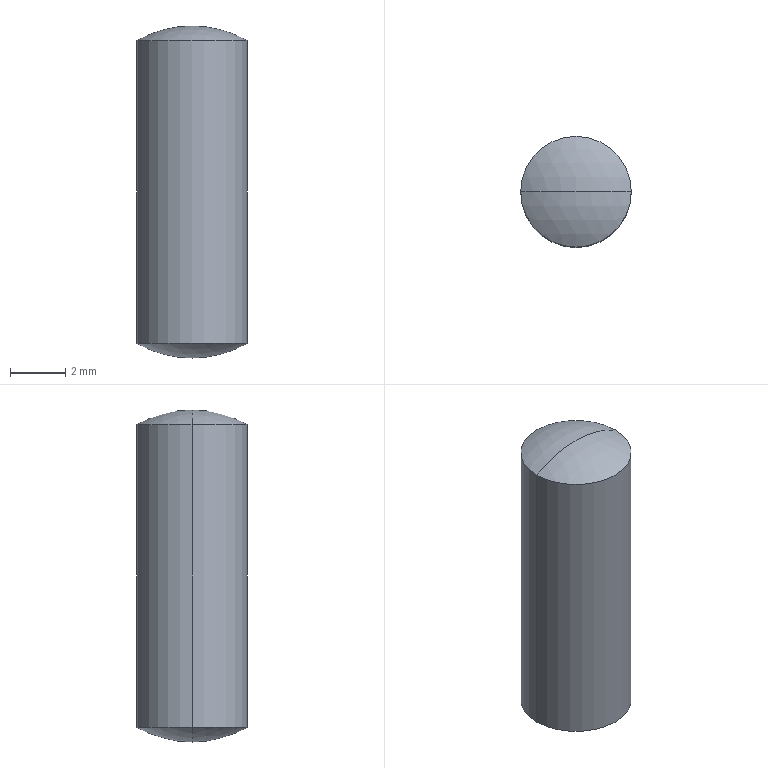Part | SolidWorks | features Attribute 1, Revolution 1 | 1 solid | 6 faces | box 4 x 4 x 12 mm | volume 144.223 mm3 | sphere 4 | cylinder 2 | commonest cylinder face diameters 4 x2
STEP:
#1=CARTESIAN_POINT('',(-2.,0.,3.464));
#2=VERTEX_POINT('',#1);
#3=CARTESIAN_POINT('',(2.,0.,3.464));
#4=VERTEX_POINT('',#3);
#5=CARTESIAN_POINT('',(0.,0.,3.464));
#6=DIRECTION('',(0.,0.,-1.));
#7=DIRECTION('',(-1.,0.,0.));
#8=AXIS2_PLACEMENT_3D('',#5,#6,#7);
#9=CIRCLE('',#8,2.);
#10=EDGE_CURVE('',#2,#4,#9,.T.);
#11=ORIENTED_EDGE('',*,*,#10,.T.);
#12=CARTESIAN_POINT('',(2.,0.,-7.464));
#13=VERTEX_POINT('',#12);
#14=CARTESIAN_POINT('',(2.,0.,-47.537));
#15=DIRECTION('',(0.,0.,-1.));
#16=VECTOR('',#15,1000.);
#17=LINE('',#14,#16);
#18=EDGE_CURVE('',#4,#13,#17,.T.);
#19=ORIENTED_EDGE('',*,*,#18,.T.);
#20=CARTESIAN_POINT('',(-2.,0.,-7.464));
#21=VERTEX_POINT('',#20);
#22=CARTESIAN_POINT('',(0.,0.,-7.464));
#23=DIRECTION('',(0.,0.,-1.));
#24=DIRECTION('',(-1.,0.,0.));
#25=AXIS2_PLACEMENT_3D('',#22,#23,#24);
#26=CIRCLE('',#25,2.);
#27=EDGE_CURVE('',#21,#13,#26,.T.);
#28=ORIENTED_EDGE('',*,*,#27,.F.);
#29=CARTESIAN_POINT('',(-2.,0.,-47.537));
#30=DIRECTION('',(0.,0.,-1.));
#31=VECTOR('',#30,1000.);
#32=LINE('',#29,#31);
#33=EDGE_CURVE('',#2,#21,#32,.T.);
#34=ORIENTED_EDGE('',*,*,#33,.F.);
#35=EDGE_LOOP('',(#11,#19,#28,#34));
#36=FACE_OUTER_BOUND('',#35,.T.);
#37=CARTESIAN_POINT('',(0.,0.,-47.537));
#38=DIRECTION('',(0.,0.,-1.));
#39=DIRECTION('',(-1.,0.,0.));
#40=AXIS2_PLACEMENT_3D('',#37,#38,#39);
#41=CYLINDRICAL_SURFACE('',#40,2.);
#42=ADVANCED_FACE('',(#36),#41,.T.);
#43=CARTESIAN_POINT('',(0.,0.,4.));
#44=VERTEX_POINT('',#43);
#45=CARTESIAN_POINT('',(0.,0.,0.));
#46=DIRECTION('',(0.,1.,0.));
#47=DIRECTION('',(0.,0.,1.));
#48=AXIS2_PLACEMENT_3D('',#45,#46,#47);
#49=CIRCLE('',#48,4.);
#50=EDGE_CURVE('',#44,#4,#49,.T.);
#51=ORIENTED_EDGE('',*,*,#50,.F.);
#52=CARTESIAN_POINT('',(0.,0.,0.));
#53=DIRECTION('',(0.,-1.,0.));
#54=DIRECTION('',(1.,0.,0.));
#55=AXIS2_PLACEMENT_3D('',#52,#53,#54);
#56=CIRCLE('',#55,4.);
#57=EDGE_CURVE('',#44,#2,#56,.T.);
#58=ORIENTED_EDGE('',*,*,#57,.T.);
#59=CARTESIAN_POINT('',(0.,0.,3.464));
#60=DIRECTION('',(0.,0.,-1.));
#61=DIRECTION('',(-1.,0.,0.));
#62=AXIS2_PLACEMENT_3D('',#59,#60,#61);
#63=CIRCLE('',#62,2.);
#64=EDGE_CURVE('',#4,#2,#63,.T.);
#65=ORIENTED_EDGE('',*,*,#64,.F.);
#66=EDGE_LOOP('',(#51,#58,#65));
#67=FACE_OUTER_BOUND('',#66,.T.);
#68=CARTESIAN_POINT('',(0.,0.,0.));
#69=DIRECTION('',(0.,-1.,0.));
#70=DIRECTION('',(1.,0.,0.));
#71=AXIS2_PLACEMENT_3D('',#68,#69,#70);
#72=SPHERICAL_SURFACE('',#71,4.);
#73=ADVANCED_FACE('',(#67),#72,.T.);
#74=ORIENTED_EDGE('',*,*,#27,.T.);
#75=CARTESIAN_POINT('',(0.,0.,-8.));
#76=VERTEX_POINT('',#75);
#77=CARTESIAN_POINT('',(0.,0.,-4.));
#78=DIRECTION('',(0.,1.,0.));
#79=DIRECTION('',(-1.,0.,0.));
#80=AXIS2_PLACEMENT_3D('',#77,#78,#79);
#81=CIRCLE('',#80,4.);
#82=EDGE_CURVE('',#13,#76,#81,.T.);
#83=ORIENTED_EDGE('',*,*,#82,.T.);
#84=CARTESIAN_POINT('',(0.,0.,-4.));
#85=DIRECTION('',(0.,-1.,0.));
#86=DIRECTION('',(0.,0.,-1.));
#87=AXIS2_PLACEMENT_3D('',#84,#85,#86);
#88=CIRCLE('',#87,4.);
#89=EDGE_CURVE('',#21,#76,#88,.T.);
#90=ORIENTED_EDGE('',*,*,#89,.F.);
#91=EDGE_LOOP('',(#74,#83,#90));
#92=FACE_OUTER_BOUND('',#91,.T.);
#93=CARTESIAN_POINT('',(0.,0.,-4.));
#94=DIRECTION('',(0.,1.,0.));
#95=DIRECTION('',(-1.,0.,0.));
#96=AXIS2_PLACEMENT_3D('',#93,#94,#95);
#97=SPHERICAL_SURFACE('',#96,4.);
#98=ADVANCED_FACE('',(#92),#97,.T.);
#99=ORIENTED_EDGE('',*,*,#82,.F.);
#100=CARTESIAN_POINT('',(0.,0.,-7.464));
#101=DIRECTION('',(0.,0.,-1.));
#102=DIRECTION('',(-1.,0.,0.));
#103=AXIS2_PLACEMENT_3D('',#100,#101,#102);
#104=CIRCLE('',#103,2.);
#105=EDGE_CURVE('',#13,#21,#104,.T.);
#106=ORIENTED_EDGE('',*,*,#105,.T.);
#107=ORIENTED_EDGE('',*,*,#89,.T.);
#108=EDGE_LOOP('',(#99,#106,#107));
#109=FACE_OUTER_BOUND('',#108,.T.);
#110=CARTESIAN_POINT('',(0.,0.,-4.));
#111=DIRECTION('',(0.,1.,0.));
#112=DIRECTION('',(-1.,0.,0.));
#113=AXIS2_PLACEMENT_3D('',#110,#111,#112);
#114=SPHERICAL_SURFACE('',#113,4.);
#115=ADVANCED_FACE('',(#109),#114,.T.);
#116=ORIENTED_EDGE('',*,*,#57,.F.);
#117=ORIENTED_EDGE('',*,*,#50,.T.);
#118=ORIENTED_EDGE('',*,*,#10,.F.);
#119=EDGE_LOOP('',(#116,#117,#118));
#120=FACE_OUTER_BOUND('',#119,.T.);
#121=CARTESIAN_POINT('',(0.,0.,0.));
#122=DIRECTION('',(0.,-1.,0.));
#123=DIRECTION('',(1.,0.,0.));
#124=AXIS2_PLACEMENT_3D('',#121,#122,#123);
#125=SPHERICAL_SURFACE('',#124,4.);
#126=ADVANCED_FACE('',(#120),#125,.T.);
#127=ORIENTED_EDGE('',*,*,#18,.F.);
#128=ORIENTED_EDGE('',*,*,#64,.T.);
#129=ORIENTED_EDGE('',*,*,#33,.T.);
#130=ORIENTED_EDGE('',*,*,#105,.F.);
#131=EDGE_LOOP('',(#127,#128,#129,#130));
#132=FACE_OUTER_BOUND('',#131,.T.);
#133=CARTESIAN_POINT('',(0.,0.,-47.537));
#134=DIRECTION('',(0.,0.,-1.));
#135=DIRECTION('',(-1.,0.,0.));
#136=AXIS2_PLACEMENT_3D('',#133,#134,#135);
#137=CYLINDRICAL_SURFACE('',#136,2.);
#138=ADVANCED_FACE('',(#132),#137,.T.);
#139=CLOSED_SHELL('',(#42,#73,#98,#115,#126,#138));
#140=MANIFOLD_SOLID_BREP('',#139);
#141=CARTESIAN_POINT('',(0.,0.,0.));
#142=DIRECTION('',(0.,0.,1.));
#143=DIRECTION('',(1.,0.,0.));
#144=AXIS2_PLACEMENT_3D('',#141,#142,#143);
#145=(LENGTH_UNIT()NAMED_UNIT(*)SI_UNIT(.MILLI.,.METRE.));
#146=UNCERTAINTY_MEASURE_WITH_UNIT(LENGTH_MEASURE(0.00001),#145,'','');
#147=(NAMED_UNIT(*)PLANE_ANGLE_UNIT()SI_UNIT($,.RADIAN.));
#148=(NAMED_UNIT(*)SI_UNIT($,.STERADIAN.)SOLID_ANGLE_UNIT());
#149=(GEOMETRIC_REPRESENTATION_CONTEXT(3)GLOBAL_UNCERTAINTY_ASSIGNED_CONTEXT((#146))GLOBAL_UNIT_ASSIGNED_CONTEXT((#145,#147,#148))REPRESENTATION_CONTEXT('',''));
#150=ADVANCED_BREP_SHAPE_REPRESENTATION('',(#140,#144),#149);